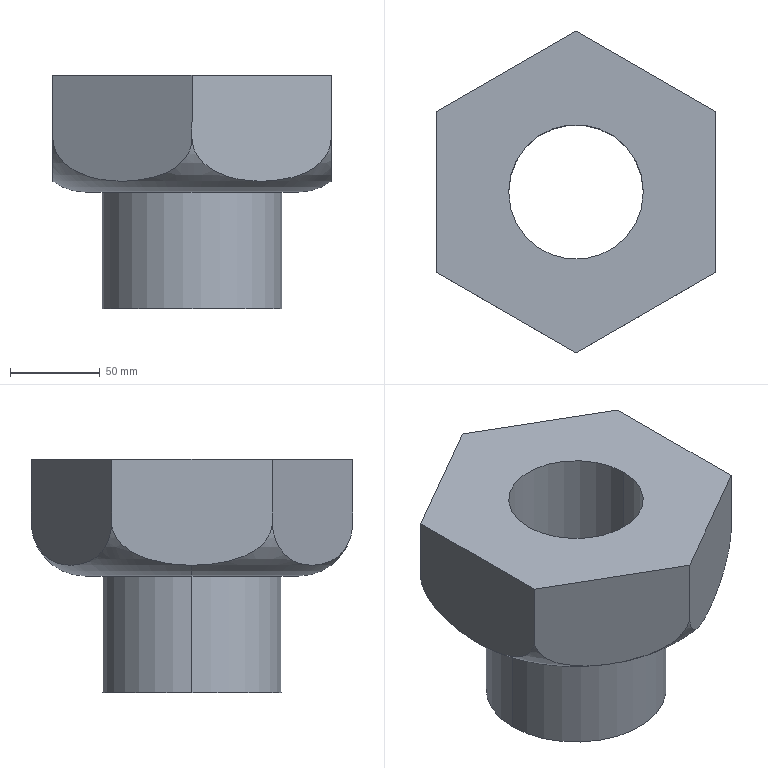Part | SolidWorks | features ICE 2, Extrusion 1, RevCut 1 | 1 solid | 15 faces | box 155 x 178.979 x 130 mm | volume 1254035 mm3 | plane 9 | cylinder 4 | torus 2 | commonest cylinder face diameters 75 x2 100 x2
STEP:
#1=CARTESIAN_POINT('',(37.5,0.,-65.));
#2=VERTEX_POINT('',#1);
#3=CARTESIAN_POINT('',(-37.5,0.,-65.));
#4=VERTEX_POINT('',#3);
#5=CARTESIAN_POINT('',(0.,0.,-65.));
#6=DIRECTION('',(0.,0.,-1.));
#7=DIRECTION('',(-1.,0.,0.));
#8=AXIS2_PLACEMENT_3D('',#5,#6,#7);
#9=CIRCLE('',#8,37.5);
#10=EDGE_CURVE('',#2,#4,#9,.T.);
#11=ORIENTED_EDGE('',*,*,#10,.T.);
#12=CARTESIAN_POINT('',(-37.5,0.,65.));
#13=VERTEX_POINT('',#12);
#14=CARTESIAN_POINT('',(-37.5,0.,-65.));
#15=DIRECTION('',(0.,0.,1.));
#16=VECTOR('',#15,1000.);
#17=LINE('',#14,#16);
#18=EDGE_CURVE('',#4,#13,#17,.T.);
#19=ORIENTED_EDGE('',*,*,#18,.T.);
#20=CARTESIAN_POINT('',(37.5,0.,65.));
#21=VERTEX_POINT('',#20);
#22=CARTESIAN_POINT('',(0.,0.,65.));
#23=DIRECTION('',(0.,0.,1.));
#24=DIRECTION('',(1.,0.,0.));
#25=AXIS2_PLACEMENT_3D('',#22,#23,#24);
#26=CIRCLE('',#25,37.5);
#27=EDGE_CURVE('',#13,#21,#26,.T.);
#28=ORIENTED_EDGE('',*,*,#27,.T.);
#29=CARTESIAN_POINT('',(37.5,0.,-65.));
#30=DIRECTION('',(0.,0.,1.));
#31=VECTOR('',#30,1000.);
#32=LINE('',#29,#31);
#33=EDGE_CURVE('',#2,#21,#32,.T.);
#34=ORIENTED_EDGE('',*,*,#33,.F.);
#35=EDGE_LOOP('',(#11,#19,#28,#34));
#36=FACE_OUTER_BOUND('',#35,.T.);
#37=CARTESIAN_POINT('',(0.,0.,-65.));
#38=DIRECTION('',(0.,0.,1.));
#39=DIRECTION('',(1.,0.,0.));
#40=AXIS2_PLACEMENT_3D('',#37,#38,#39);
#41=CYLINDRICAL_SURFACE('',#40,37.5);
#42=ADVANCED_FACE('',(#36),#41,.F.);
#43=CARTESIAN_POINT('',(-50.,0.,-65.));
#44=VERTEX_POINT('',#43);
#45=CARTESIAN_POINT('',(50.,0.,-65.));
#46=VERTEX_POINT('',#45);
#47=CARTESIAN_POINT('',(0.,0.,-65.));
#48=DIRECTION('',(0.,0.,-1.));
#49=DIRECTION('',(-1.,0.,0.));
#50=AXIS2_PLACEMENT_3D('',#47,#48,#49);
#51=CIRCLE('',#50,50.);
#52=EDGE_CURVE('',#44,#46,#51,.T.);
#53=ORIENTED_EDGE('',*,*,#52,.F.);
#54=CARTESIAN_POINT('',(-50.,0.,0.));
#55=VERTEX_POINT('',#54);
#56=CARTESIAN_POINT('',(-50.,0.,-65.));
#57=DIRECTION('',(0.,0.,1.));
#58=VECTOR('',#57,1000.);
#59=LINE('',#56,#58);
#60=EDGE_CURVE('',#44,#55,#59,.T.);
#61=ORIENTED_EDGE('',*,*,#60,.T.);
#62=CARTESIAN_POINT('',(50.,0.,0.));
#63=VERTEX_POINT('',#62);
#64=CARTESIAN_POINT('',(0.,0.,0.));
#65=DIRECTION('',(0.,0.,-1.));
#66=DIRECTION('',(1.,0.,0.));
#67=AXIS2_PLACEMENT_3D('',#64,#65,#66);
#68=CIRCLE('',#67,50.);
#69=EDGE_CURVE('',#55,#63,#68,.T.);
#70=ORIENTED_EDGE('',*,*,#69,.T.);
#71=CARTESIAN_POINT('',(50.,0.,-65.));
#72=DIRECTION('',(0.,0.,1.));
#73=VECTOR('',#72,1000.);
#74=LINE('',#71,#73);
#75=EDGE_CURVE('',#46,#63,#74,.T.);
#76=ORIENTED_EDGE('',*,*,#75,.F.);
#77=EDGE_LOOP('',(#53,#61,#70,#76));
#78=FACE_OUTER_BOUND('',#77,.T.);
#79=CARTESIAN_POINT('',(0.,0.,-65.));
#80=DIRECTION('',(0.,0.,1.));
#81=DIRECTION('',(1.,0.,0.));
#82=AXIS2_PLACEMENT_3D('',#79,#80,#81);
#83=CYLINDRICAL_SURFACE('',#82,50.);
#84=ADVANCED_FACE('',(#78),#83,.T.);
#85=CARTESIAN_POINT('',(59.489,0.,0.));
#86=VERTEX_POINT('',#85);
#87=CARTESIAN_POINT('',(-59.489,0.,0.));
#88=VERTEX_POINT('',#87);
#89=CARTESIAN_POINT('',(0.,0.,0.));
#90=DIRECTION('',(0.,0.,1.));
#91=DIRECTION('',(1.,0.,0.));
#92=AXIS2_PLACEMENT_3D('',#89,#90,#91);
#93=CIRCLE('',#92,59.489);
#94=EDGE_CURVE('',#86,#88,#93,.T.);
#95=ORIENTED_EDGE('',*,*,#94,.T.);
#96=CARTESIAN_POINT('',(-77.5,0.,6.008));
#97=VERTEX_POINT('',#96);
#98=CARTESIAN_POINT('',(-59.489,0.,30.));
#99=DIRECTION('',(0.,1.,0.));
#100=DIRECTION('',(-1.,0.,0.));
#101=AXIS2_PLACEMENT_3D('',#98,#99,#100);
#102=CIRCLE('',#101,30.);
#103=EDGE_CURVE('',#88,#97,#102,.T.);
#104=ORIENTED_EDGE('',*,*,#103,.T.);
#105=CARTESIAN_POINT('',(-77.5,44.745,30.));
#106=VERTEX_POINT('',#105);
#107=CARTESIAN_POINT('',(-77.5,0.,6.008));
#108=CARTESIAN_POINT('',(-77.5,2.326,6.008));
#109=CARTESIAN_POINT('',(-77.5,4.641,6.086));
#110=CARTESIAN_POINT('',(-77.5,9.25,6.403));
#111=CARTESIAN_POINT('',(-77.5,11.544,6.643));
#112=CARTESIAN_POINT('',(-77.5,16.107,7.312));
#113=CARTESIAN_POINT('',(-77.5,18.376,7.742));
#114=CARTESIAN_POINT('',(-77.5,21.755,8.571));
#115=CARTESIAN_POINT('',(-77.5,22.878,8.879));
#116=CARTESIAN_POINT('',(-77.5,25.11,9.566));
#117=CARTESIAN_POINT('',(-77.5,26.212,9.944));
#118=CARTESIAN_POINT('',(-77.5,28.383,10.777));
#119=CARTESIAN_POINT('',(-77.5,29.453,11.232));
#120=CARTESIAN_POINT('',(-77.5,31.028,11.984));
#121=CARTESIAN_POINT('',(-77.5,31.548,12.246));
#122=CARTESIAN_POINT('',(-77.5,32.578,12.795));
#123=CARTESIAN_POINT('',(-77.5,33.089,13.083));
#124=CARTESIAN_POINT('',(-77.5,34.59,13.98));
#125=CARTESIAN_POINT('',(-77.5,35.553,14.624));
#126=CARTESIAN_POINT('',(-77.5,37.393,16.021));
#127=CARTESIAN_POINT('',(-77.5,38.27,16.773));
#128=CARTESIAN_POINT('',(-77.5,39.506,17.998));
#129=CARTESIAN_POINT('',(-77.5,39.905,18.422));
#130=CARTESIAN_POINT('',(-77.5,40.673,19.309));
#131=CARTESIAN_POINT('',(-77.5,41.04,19.769));
#132=CARTESIAN_POINT('',(-77.5,42.074,21.184));
#133=CARTESIAN_POINT('',(-77.5,42.676,22.179));
#134=CARTESIAN_POINT('',(-77.5,43.43,23.763));
#135=CARTESIAN_POINT('',(-77.5,43.657,24.31));
#136=CARTESIAN_POINT('',(-77.5,44.047,25.415));
#137=CARTESIAN_POINT('',(-77.5,44.21,25.973));
#138=CARTESIAN_POINT('',(-77.5,44.607,27.667));
#139=CARTESIAN_POINT('',(-77.5,44.745,28.82));
#140=CARTESIAN_POINT('',(-77.5,44.745,30.));
#141=B_SPLINE_CURVE_WITH_KNOTS('',3,(#107,#108,#109,#110,#111,#112,#113,#114,#115,#116,#117,#118,#119,#120,#121,#122,#123,#124,#125,#126,#127,#128,#129,#130,#131,#132,#133,#134,#135,#136,#137,#138,#139,#140),.UNSPECIFIED.,.F.,.F.,(4,2,2,2,2,2,2,2,2,2,2,2,2,2,2,2,4),(0.,0.006917,0.01383,0.02075,0.02421,0.02767,0.03113,0.03285,0.03458,0.03804,0.0415,0.04323,0.04496,0.04842,0.05015,0.05188,0.05533),.UNSPECIFIED.);
#142=EDGE_CURVE('',#97,#106,#141,.T.);
#143=ORIENTED_EDGE('',*,*,#142,.T.);
#144=CARTESIAN_POINT('',(0.,89.489,30.));
#145=VERTEX_POINT('',#144);
#146=CARTESIAN_POINT('',(-77.5,44.745,30.));
#147=CARTESIAN_POINT('',(-77.5,44.745,28.82));
#148=CARTESIAN_POINT('',(-77.38,44.814,27.664));
#149=CARTESIAN_POINT('',(-77.035,45.013,25.963));
#150=CARTESIAN_POINT('',(-76.892,45.096,25.402));
#151=CARTESIAN_POINT('',(-76.551,45.292,24.291));
#152=CARTESIAN_POINT('',(-76.356,45.405,23.75));
#153=CARTESIAN_POINT('',(-75.704,45.782,22.169));
#154=CARTESIAN_POINT('',(-75.18,46.084,21.171));
#155=CARTESIAN_POINT('',(-73.975,46.78,19.271));
#156=CARTESIAN_POINT('',(-73.311,47.163,18.395));
#157=CARTESIAN_POINT('',(-71.883,47.988,16.763));
#158=CARTESIAN_POINT('',(-71.119,48.429,16.007));
#159=CARTESIAN_POINT('',(-69.909,49.127,14.949));
#160=CARTESIAN_POINT('',(-69.494,49.367,14.608));
#161=CARTESIAN_POINT('',(-68.653,49.852,13.958));
#162=CARTESIAN_POINT('',(-68.227,50.099,13.648));
#163=CARTESIAN_POINT('',(-66.066,51.346,12.163));
#164=CARTESIAN_POINT('',(-64.251,52.394,11.184));
#165=CARTESIAN_POINT('',(-61.436,54.019,9.938));
#166=CARTESIAN_POINT('',(-60.479,54.571,9.56));
#167=CARTESIAN_POINT('',(-58.55,55.686,8.874));
#168=CARTESIAN_POINT('',(-57.58,56.245,8.568));
#169=CARTESIAN_POINT('',(-54.66,57.931,7.741));
#170=CARTESIAN_POINT('',(-52.697,59.064,7.312));
#171=CARTESIAN_POINT('',(-48.749,61.344,6.643));
#172=CARTESIAN_POINT('',(-46.763,62.491,6.403));
#173=CARTESIAN_POINT('',(-43.769,64.22,6.165));
#174=CARTESIAN_POINT('',(-42.768,64.797,6.106));
#175=CARTESIAN_POINT('',(-40.761,65.956,6.028));
#176=CARTESIAN_POINT('',(-39.754,66.537,6.008));
#177=CARTESIAN_POINT('',(-36.741,68.277,6.008));
#178=CARTESIAN_POINT('',(-34.74,69.432,6.085));
#179=CARTESIAN_POINT('',(-30.759,71.731,6.401));
#180=CARTESIAN_POINT('',(-28.777,72.875,6.639));
#181=CARTESIAN_POINT('',(-24.836,75.15,7.305));
#182=CARTESIAN_POINT('',(-22.877,76.282,7.732));
#183=CARTESIAN_POINT('',(-19.958,77.966,8.556));
#184=CARTESIAN_POINT('',(-18.989,78.526,8.862));
#185=CARTESIAN_POINT('',(-17.059,79.64,9.545));
#186=CARTESIAN_POINT('',(-16.099,80.195,9.924));
#187=CARTESIAN_POINT('',(-14.213,81.284,10.756));
#188=CARTESIAN_POINT('',(-13.285,81.819,11.211));
#189=CARTESIAN_POINT('',(-11.918,82.608,11.961));
#190=CARTESIAN_POINT('',(-11.467,82.869,12.223));
#191=CARTESIAN_POINT('',(-10.574,83.385,12.771));
#192=CARTESIAN_POINT('',(-10.131,83.64,13.058));
#193=CARTESIAN_POINT('',(-8.827,84.393,13.955));
#194=CARTESIAN_POINT('',(-7.99,84.876,14.6));
#195=CARTESIAN_POINT('',(-6.389,85.8,15.999));
#196=CARTESIAN_POINT('',(-5.626,86.241,16.753));
#197=CARTESIAN_POINT('',(-4.549,86.863,17.983));
#198=CARTESIAN_POINT('',(-4.2,87.064,18.411));
#199=CARTESIAN_POINT('',(-3.535,87.448,19.297));
#200=CARTESIAN_POINT('',(-3.219,87.631,19.753));
#201=CARTESIAN_POINT('',(-2.326,88.146,21.162));
#202=CARTESIAN_POINT('',(-1.802,88.449,22.156));
#203=CARTESIAN_POINT('',(-1.146,88.828,23.745));
#204=CARTESIAN_POINT('',(-0.9494,88.941,24.289));
#205=CARTESIAN_POINT('',(-0.6116,89.136,25.389));
#206=CARTESIAN_POINT('',(-0.4689,89.219,25.947));
#207=CARTESIAN_POINT('',(-0.2379,89.352,27.079));
#208=CARTESIAN_POINT('',(-0.1495,89.403,27.653));
#209=CARTESIAN_POINT('',(-0.03038,89.472,28.819));
#210=CARTESIAN_POINT('',(0.,89.489,29.41));
#211=CARTESIAN_POINT('',(0.,89.489,30.));
#212=B_SPLINE_CURVE_WITH_KNOTS('',3,(#146,#147,#148,#149,#150,#151,#152,#153,#154,#155,#156,#157,#158,#159,#160,#161,#162,#163,#164,#165,#166,#167,#168,#169,#170,#171,#172,#173,#174,#175,#176,#177,#178,#179,#180,#181,#182,#183,#184,#185,#186,#187,#188,#189,#190,#191,#192,#193,#194,#195,#196,#197,#198,#199,#200,#201,#202,#203,#204,#205,#206,#207,#208,#209,#210,#211),.UNSPECIFIED.,.F.,.F.,(4,2,2,2,2,2,2,2,2,2,2,2,2,2,2,2,2,2,2,2,2,2,2,2,2,2,2,2,2,2,2,2,4),(0.000000197,0.003488,0.005232,0.006975,0.01046,0.01395,0.01744,0.01918,0.02093,0.0279,0.03139,0.03488,0.04185,0.04883,0.05231,0.0558,0.06278,0.06975,0.07673,0.08021,0.0837,0.08719,0.08893,0.09068,0.09417,0.09765,0.0994,0.1011,0.1046,0.1064,0.1081,0.1099,0.1116),.UNSPECIFIED.);
#213=EDGE_CURVE('',#106,#145,#212,.T.);
#214=ORIENTED_EDGE('',*,*,#213,.T.);
#215=CARTESIAN_POINT('',(77.5,44.745,30.));
#216=VERTEX_POINT('',#215);
#217=CARTESIAN_POINT('',(0.,89.489,30.));
#218=CARTESIAN_POINT('',(0.,89.489,28.82));
#219=CARTESIAN_POINT('',(0.1197,89.42,27.664));
#220=CARTESIAN_POINT('',(0.465,89.221,25.963));
#221=CARTESIAN_POINT('',(0.6079,89.138,25.402));
#222=CARTESIAN_POINT('',(0.9488,88.942,24.291));
#223=CARTESIAN_POINT('',(1.144,88.829,23.75));
#224=CARTESIAN_POINT('',(1.796,88.452,22.169));
#225=CARTESIAN_POINT('',(2.32,88.15,21.171));
#226=CARTESIAN_POINT('',(3.525,87.454,19.271));
#227=CARTESIAN_POINT('',(4.189,87.071,18.395));
#228=CARTESIAN_POINT('',(5.617,86.246,16.763));
#229=CARTESIAN_POINT('',(6.381,85.805,16.007));
#230=CARTESIAN_POINT('',(7.591,85.107,14.949));
#231=CARTESIAN_POINT('',(8.006,84.867,14.608));
#232=CARTESIAN_POINT('',(8.847,84.382,13.958));
#233=CARTESIAN_POINT('',(9.273,84.135,13.648));
#234=CARTESIAN_POINT('',(11.434,82.888,12.163));
#235=CARTESIAN_POINT('',(13.249,81.84,11.184));
#236=CARTESIAN_POINT('',(16.064,80.215,9.938));
#237=CARTESIAN_POINT('',(17.021,79.662,9.56));
#238=CARTESIAN_POINT('',(18.95,78.548,8.874));
#239=CARTESIAN_POINT('',(19.92,77.988,8.568));
#240=CARTESIAN_POINT('',(22.84,76.302,7.741));
#241=CARTESIAN_POINT('',(24.803,75.17,7.312));
#242=CARTESIAN_POINT('',(28.751,72.89,6.643));
#243=CARTESIAN_POINT('',(30.737,71.743,6.403));
#244=CARTESIAN_POINT('',(33.731,70.014,6.165));
#245=CARTESIAN_POINT('',(34.732,69.437,6.106));
#246=CARTESIAN_POINT('',(36.739,68.278,6.028));
#247=CARTESIAN_POINT('',(37.746,67.697,6.008));
#248=CARTESIAN_POINT('',(40.759,65.957,6.008));
#249=CARTESIAN_POINT('',(42.76,64.802,6.085));
#250=CARTESIAN_POINT('',(46.741,62.503,6.401));
#251=CARTESIAN_POINT('',(48.723,61.359,6.639));
#252=CARTESIAN_POINT('',(52.664,59.084,7.305));
#253=CARTESIAN_POINT('',(54.623,57.952,7.732));
#254=CARTESIAN_POINT('',(57.542,56.268,8.556));
#255=CARTESIAN_POINT('',(58.511,55.708,8.862));
#256=CARTESIAN_POINT('',(60.441,54.594,9.545));
#257=CARTESIAN_POINT('',(61.401,54.039,9.924));
#258=CARTESIAN_POINT('',(63.287,52.95,10.756));
#259=CARTESIAN_POINT('',(64.215,52.415,11.211));
#260=CARTESIAN_POINT('',(65.582,51.625,11.961));
#261=CARTESIAN_POINT('',(66.033,51.365,12.223));
#262=CARTESIAN_POINT('',(66.926,50.849,12.771));
#263=CARTESIAN_POINT('',(67.369,50.594,13.058));
#264=CARTESIAN_POINT('',(68.673,49.841,13.955));
#265=CARTESIAN_POINT('',(69.51,49.358,14.6));
#266=CARTESIAN_POINT('',(71.111,48.434,15.999));
#267=CARTESIAN_POINT('',(71.874,47.993,16.753));
#268=CARTESIAN_POINT('',(72.951,47.371,17.983));
#269=CARTESIAN_POINT('',(73.3,47.17,18.411));
#270=CARTESIAN_POINT('',(73.965,46.786,19.297));
#271=CARTESIAN_POINT('',(74.281,46.603,19.753));
#272=CARTESIAN_POINT('',(75.174,46.088,21.162));
#273=CARTESIAN_POINT('',(75.698,45.785,22.156));
#274=CARTESIAN_POINT('',(76.354,45.406,23.745));
#275=CARTESIAN_POINT('',(76.551,45.293,24.289));
#276=CARTESIAN_POINT('',(76.888,45.098,25.389));
#277=CARTESIAN_POINT('',(77.031,45.015,25.947));
#278=CARTESIAN_POINT('',(77.262,44.882,27.079));
#279=CARTESIAN_POINT('',(77.35,44.831,27.653));
#280=CARTESIAN_POINT('',(77.47,44.762,28.819));
#281=CARTESIAN_POINT('',(77.5,44.745,29.41));
#282=CARTESIAN_POINT('',(77.5,44.745,30.));
#283=B_SPLINE_CURVE_WITH_KNOTS('',3,(#217,#218,#219,#220,#221,#222,#223,#224,#225,#226,#227,#228,#229,#230,#231,#232,#233,#234,#235,#236,#237,#238,#239,#240,#241,#242,#243,#244,#245,#246,#247,#248,#249,#250,#251,#252,#253,#254,#255,#256,#257,#258,#259,#260,#261,#262,#263,#264,#265,#266,#267,#268,#269,#270,#271,#272,#273,#274,#275,#276,#277,#278,#279,#280,#281,#282),.UNSPECIFIED.,.F.,.F.,(4,2,2,2,2,2,2,2,2,2,2,2,2,2,2,2,2,2,2,2,2,2,2,2,2,2,2,2,2,2,2,2,4),(0.000000197,0.003488,0.005232,0.006975,0.01046,0.01395,0.01744,0.01918,0.02093,0.0279,0.03139,0.03488,0.04185,0.04883,0.05231,0.0558,0.06278,0.06975,0.07673,0.08021,0.0837,0.08719,0.08893,0.09068,0.09417,0.09765,0.0994,0.1011,0.1046,0.1064,0.1081,0.1099,0.1116),.UNSPECIFIED.);
#284=EDGE_CURVE('',#145,#216,#283,.T.);
#285=ORIENTED_EDGE('',*,*,#284,.T.);
#286=CARTESIAN_POINT('',(77.5,0.,6.008));
#287=VERTEX_POINT('',#286);
#288=CARTESIAN_POINT('',(77.5,44.745,30.));
#289=CARTESIAN_POINT('',(77.5,44.745,29.421));
#290=CARTESIAN_POINT('',(77.5,44.711,28.842));
#291=CARTESIAN_POINT('',(77.5,44.576,27.68));
#292=CARTESIAN_POINT('',(77.5,44.474,27.097));
#293=CARTESIAN_POINT('',(77.5,44.073,25.391));
#294=CARTESIAN_POINT('',(77.5,43.682,24.295));
#295=CARTESIAN_POINT('',(77.5,42.927,22.706));
#296=CARTESIAN_POINT('',(77.5,42.647,22.187));
#297=CARTESIAN_POINT('',(77.5,42.046,21.188));
#298=CARTESIAN_POINT('',(77.5,41.724,20.705));
#299=CARTESIAN_POINT('',(77.5,40.698,19.3));
#300=CARTESIAN_POINT('',(77.5,39.934,18.423));
#301=CARTESIAN_POINT('',(77.5,38.686,17.185));
#302=CARTESIAN_POINT('',(77.5,38.255,16.788));
#303=CARTESIAN_POINT('',(77.5,37.374,16.028));
#304=CARTESIAN_POINT('',(77.5,36.923,15.663));
#305=CARTESIAN_POINT('',(77.5,35.538,14.614));
#306=CARTESIAN_POINT('',(77.5,34.576,13.971));
#307=CARTESIAN_POINT('',(77.5,33.084,13.08));
#308=CARTESIAN_POINT('',(77.5,32.578,12.795));
#309=CARTESIAN_POINT('',(77.5,31.551,12.247));
#310=CARTESIAN_POINT('',(77.5,31.028,11.984));
#311=CARTESIAN_POINT('',(77.5,29.449,11.23));
#312=CARTESIAN_POINT('',(77.5,28.381,10.776));
#313=CARTESIAN_POINT('',(77.5,25.143,9.533));
#314=CARTESIAN_POINT('',(77.5,22.936,8.863));
#315=CARTESIAN_POINT('',(77.5,19.574,8.034));
#316=CARTESIAN_POINT('',(77.5,18.445,7.788));
#317=CARTESIAN_POINT('',(77.5,16.17,7.348));
#318=CARTESIAN_POINT('',(77.5,15.023,7.154));
#319=CARTESIAN_POINT('',(77.5,11.575,6.646));
#320=CARTESIAN_POINT('',(77.5,9.268,6.405));
#321=CARTESIAN_POINT('',(77.5,5.8,6.165));
#322=CARTESIAN_POINT('',(77.5,4.642,6.106));
#323=CARTESIAN_POINT('',(77.5,2.903,6.047));
#324=CARTESIAN_POINT('',(77.5,2.323,6.033));
#325=CARTESIAN_POINT('',(77.5,1.452,6.018));
#326=CARTESIAN_POINT('',(77.5,1.162,6.014));
#327=CARTESIAN_POINT('',(77.5,0.5811,6.009));
#328=CARTESIAN_POINT('',(77.5,0.2891,6.008));
#329=CARTESIAN_POINT('',(77.5,0.,6.008));
#330=B_SPLINE_CURVE_WITH_KNOTS('',3,(#288,#289,#290,#291,#292,#293,#294,#295,#296,#297,#298,#299,#300,#301,#302,#303,#304,#305,#306,#307,#308,#309,#310,#311,#312,#313,#314,#315,#316,#317,#318,#319,#320,#321,#322,#323,#324,#325,#326,#327,#328,#329),.UNSPECIFIED.,.F.,.F.,(4,2,2,2,2,2,2,2,2,2,2,2,2,2,2,2,2,2,2,2,4),(0.1659,0.1677,0.1694,0.1728,0.1745,0.1763,0.1797,0.1814,0.1831,0.1866,0.1883,0.19,0.1935,0.2003,0.2038,0.2072,0.2141,0.2175,0.2192,0.2201,0.221),.UNSPECIFIED.);
#331=EDGE_CURVE('',#216,#287,#330,.T.);
#332=ORIENTED_EDGE('',*,*,#331,.T.);
#333=CARTESIAN_POINT('',(59.489,0.,30.));
#334=DIRECTION('',(0.,-1.,0.));
#335=DIRECTION('',(0.,0.,-1.));
#336=AXIS2_PLACEMENT_3D('',#333,#334,#335);
#337=CIRCLE('',#336,30.);
#338=EDGE_CURVE('',#86,#287,#337,.T.);
#339=ORIENTED_EDGE('',*,*,#338,.F.);
#340=EDGE_LOOP('',(#95,#104,#143,#214,#285,#332,#339));
#341=FACE_OUTER_BOUND('',#340,.T.);
#342=CARTESIAN_POINT('',(0.,0.,30.));
#343=DIRECTION('',(0.,0.,1.));
#344=DIRECTION('',(1.,0.,0.));
#345=AXIS2_PLACEMENT_3D('',#342,#343,#344);
#346=TOROIDAL_SURFACE('',#345,59.489,30.);
#347=ADVANCED_FACE('',(#341),#346,.T.);
#348=ORIENTED_EDGE('',*,*,#94,.F.);
#349=CARTESIAN_POINT('',(0.,0.,0.));
#350=DIRECTION('',(0.,0.,1.));
#351=DIRECTION('',(1.,0.,0.));
#352=AXIS2_PLACEMENT_3D('',#349,#350,#351);
#353=CIRCLE('',#352,59.489);
#354=EDGE_CURVE('',#88,#86,#353,.T.);
#355=ORIENTED_EDGE('',*,*,#354,.F.);
#356=EDGE_LOOP('',(#348,#355));
#357=FACE_OUTER_BOUND('',#356,.T.);
#358=CARTESIAN_POINT('',(0.,0.,0.));
#359=DIRECTION('',(0.,0.,-1.));
#360=DIRECTION('',(1.,0.,0.));
#361=AXIS2_PLACEMENT_3D('',#358,#359,#360);
#362=CIRCLE('',#361,50.);
#363=EDGE_CURVE('',#63,#55,#362,.T.);
#364=ORIENTED_EDGE('',*,*,#363,.F.);
#365=ORIENTED_EDGE('',*,*,#69,.F.);
#366=EDGE_LOOP('',(#364,#365));
#367=FACE_BOUND('',#366,.T.);
#368=CARTESIAN_POINT('',(0.,0.,0.));
#369=DIRECTION('',(0.,0.,1.));
#370=DIRECTION('',(1.,0.,0.));
#371=AXIS2_PLACEMENT_3D('',#368,#369,#370);
#372=PLANE('',#371);
#373=ADVANCED_FACE('',(#357,#367),#372,.F.);
#374=ORIENTED_EDGE('',*,*,#331,.F.);
#375=CARTESIAN_POINT('',(77.5,44.745,65.));
#376=VERTEX_POINT('',#375);
#377=CARTESIAN_POINT('',(77.5,44.745,65.));
#378=DIRECTION('',(0.,0.,-1.));
#379=VECTOR('',#378,1000.);
#380=LINE('',#377,#379);
#381=EDGE_CURVE('',#376,#216,#380,.T.);
#382=ORIENTED_EDGE('',*,*,#381,.F.);
#383=CARTESIAN_POINT('',(77.5,-44.745,65.));
#384=VERTEX_POINT('',#383);
#385=CARTESIAN_POINT('',(77.5,-44.745,65.));
#386=DIRECTION('',(0.,1.,0.));
#387=VECTOR('',#386,1000.);
#388=LINE('',#385,#387);
#389=EDGE_CURVE('',#384,#376,#388,.T.);
#390=ORIENTED_EDGE('',*,*,#389,.F.);
#391=CARTESIAN_POINT('',(77.5,-44.745,30.));
#392=VERTEX_POINT('',#391);
#393=CARTESIAN_POINT('',(77.5,-44.745,65.));
#394=DIRECTION('',(0.,0.,-1.));
#395=VECTOR('',#394,1000.);
#396=LINE('',#393,#395);
#397=EDGE_CURVE('',#384,#392,#396,.T.);
#398=ORIENTED_EDGE('',*,*,#397,.T.);
#399=CARTESIAN_POINT('',(77.5,0.,6.008));
#400=CARTESIAN_POINT('',(77.5,-2.326,6.008));
#401=CARTESIAN_POINT('',(77.5,-4.641,6.086));
#402=CARTESIAN_POINT('',(77.5,-9.25,6.403));
#403=CARTESIAN_POINT('',(77.5,-11.544,6.643));
#404=CARTESIAN_POINT('',(77.5,-16.107,7.312));
#405=CARTESIAN_POINT('',(77.5,-18.376,7.742));
#406=CARTESIAN_POINT('',(77.5,-21.755,8.571));
#407=CARTESIAN_POINT('',(77.5,-22.878,8.879));
#408=CARTESIAN_POINT('',(77.5,-25.11,9.566));
#409=CARTESIAN_POINT('',(77.5,-26.212,9.944));
#410=CARTESIAN_POINT('',(77.5,-28.383,10.777));
#411=CARTESIAN_POINT('',(77.5,-29.453,11.232));
#412=CARTESIAN_POINT('',(77.5,-31.028,11.984));
#413=CARTESIAN_POINT('',(77.5,-31.548,12.246));
#414=CARTESIAN_POINT('',(77.5,-32.578,12.795));
#415=CARTESIAN_POINT('',(77.5,-33.089,13.083));
#416=CARTESIAN_POINT('',(77.5,-34.59,13.98));
#417=CARTESIAN_POINT('',(77.5,-35.553,14.624));
#418=CARTESIAN_POINT('',(77.5,-37.393,16.021));
#419=CARTESIAN_POINT('',(77.5,-38.27,16.773));
#420=CARTESIAN_POINT('',(77.5,-39.506,17.998));
#421=CARTESIAN_POINT('',(77.5,-39.905,18.422));
#422=CARTESIAN_POINT('',(77.5,-40.673,19.309));
#423=CARTESIAN_POINT('',(77.5,-41.04,19.769));
#424=CARTESIAN_POINT('',(77.5,-42.074,21.184));
#425=CARTESIAN_POINT('',(77.5,-42.676,22.179));
#426=CARTESIAN_POINT('',(77.5,-43.43,23.763));
#427=CARTESIAN_POINT('',(77.5,-43.657,24.31));
#428=CARTESIAN_POINT('',(77.5,-44.047,25.415));
#429=CARTESIAN_POINT('',(77.5,-44.21,25.973));
#430=CARTESIAN_POINT('',(77.5,-44.607,27.667));
#431=CARTESIAN_POINT('',(77.5,-44.745,28.82));
#432=CARTESIAN_POINT('',(77.5,-44.745,30.));
#433=B_SPLINE_CURVE_WITH_KNOTS('',3,(#399,#400,#401,#402,#403,#404,#405,#406,#407,#408,#409,#410,#411,#412,#413,#414,#415,#416,#417,#418,#419,#420,#421,#422,#423,#424,#425,#426,#427,#428,#429,#430,#431,#432),.UNSPECIFIED.,.F.,.F.,(4,2,2,2,2,2,2,2,2,2,2,2,2,2,2,2,4),(0.,0.006917,0.01383,0.02075,0.02421,0.02767,0.03113,0.03285,0.03458,0.03804,0.0415,0.04323,0.04496,0.04842,0.05015,0.05188,0.05533),.UNSPECIFIED.);
#434=EDGE_CURVE('',#287,#392,#433,.T.);
#435=ORIENTED_EDGE('',*,*,#434,.F.);
#436=EDGE_LOOP('',(#374,#382,#390,#398,#435));
#437=FACE_OUTER_BOUND('',#436,.T.);
#438=CARTESIAN_POINT('',(77.5,-44.745,65.));
#439=DIRECTION('',(-1.,0.,0.));
#440=DIRECTION('',(0.,-1.,0.));
#441=AXIS2_PLACEMENT_3D('',#438,#439,#440);
#442=PLANE('',#441);
#443=ADVANCED_FACE('',(#437),#442,.F.);
#444=ORIENTED_EDGE('',*,*,#284,.F.);
#445=CARTESIAN_POINT('',(0.,89.489,65.));
#446=VERTEX_POINT('',#445);
#447=CARTESIAN_POINT('',(0.,89.489,65.));
#448=DIRECTION('',(0.,0.,-1.));
#449=VECTOR('',#448,1000.);
#450=LINE('',#447,#449);
#451=EDGE_CURVE('',#446,#145,#450,.T.);
#452=ORIENTED_EDGE('',*,*,#451,.F.);
#453=CARTESIAN_POINT('',(77.5,44.745,65.));
#454=DIRECTION('',(-0.866,0.5,0.));
#455=VECTOR('',#454,1000.);
#456=LINE('',#453,#455);
#457=EDGE_CURVE('',#376,#446,#456,.T.);
#458=ORIENTED_EDGE('',*,*,#457,.F.);
#459=ORIENTED_EDGE('',*,*,#381,.T.);
#460=EDGE_LOOP('',(#444,#452,#458,#459));
#461=FACE_OUTER_BOUND('',#460,.T.);
#462=CARTESIAN_POINT('',(77.5,44.745,65.));
#463=DIRECTION('',(-0.5,-0.866,0.));
#464=DIRECTION('',(0.866,-0.5,0.));
#465=AXIS2_PLACEMENT_3D('',#462,#463,#464);
#466=PLANE('',#465);
#467=ADVANCED_FACE('',(#461),#466,.F.);
#468=ORIENTED_EDGE('',*,*,#213,.F.);
#469=CARTESIAN_POINT('',(-77.5,44.745,65.));
#470=VERTEX_POINT('',#469);
#471=CARTESIAN_POINT('',(-77.5,44.745,65.));
#472=DIRECTION('',(0.,0.,-1.));
#473=VECTOR('',#472,1000.);
#474=LINE('',#471,#473);
#475=EDGE_CURVE('',#470,#106,#474,.T.);
#476=ORIENTED_EDGE('',*,*,#475,.F.);
#477=CARTESIAN_POINT('',(0.,89.489,65.));
#478=DIRECTION('',(-0.866,-0.5,0.));
#479=VECTOR('',#478,1000.);
#480=LINE('',#477,#479);
#481=EDGE_CURVE('',#446,#470,#480,.T.);
#482=ORIENTED_EDGE('',*,*,#481,.F.);
#483=ORIENTED_EDGE('',*,*,#451,.T.);
#484=EDGE_LOOP('',(#468,#476,#482,#483));
#485=FACE_OUTER_BOUND('',#484,.T.);
#486=CARTESIAN_POINT('',(0.,89.489,65.));
#487=DIRECTION('',(0.5,-0.866,0.));
#488=DIRECTION('',(0.866,0.5,0.));
#489=AXIS2_PLACEMENT_3D('',#486,#487,#488);
#490=PLANE('',#489);
#491=ADVANCED_FACE('',(#485),#490,.F.);
#492=CARTESIAN_POINT('',(-77.5,-44.745,30.));
#493=VERTEX_POINT('',#492);
#494=CARTESIAN_POINT('',(-77.5,-44.745,30.));
#495=CARTESIAN_POINT('',(-77.5,-44.745,29.421));
#496=CARTESIAN_POINT('',(-77.5,-44.711,28.842));
#497=CARTESIAN_POINT('',(-77.5,-44.576,27.68));
#498=CARTESIAN_POINT('',(-77.5,-44.474,27.097));
#499=CARTESIAN_POINT('',(-77.5,-44.073,25.391));
#500=CARTESIAN_POINT('',(-77.5,-43.682,24.295));
#501=CARTESIAN_POINT('',(-77.5,-42.927,22.706));
#502=CARTESIAN_POINT('',(-77.5,-42.647,22.187));
#503=CARTESIAN_POINT('',(-77.5,-42.046,21.188));
#504=CARTESIAN_POINT('',(-77.5,-41.724,20.705));
#505=CARTESIAN_POINT('',(-77.5,-40.698,19.3));
#506=CARTESIAN_POINT('',(-77.5,-39.934,18.423));
#507=CARTESIAN_POINT('',(-77.5,-38.686,17.185));
#508=CARTESIAN_POINT('',(-77.5,-38.255,16.788));
#509=CARTESIAN_POINT('',(-77.5,-37.374,16.028));
#510=CARTESIAN_POINT('',(-77.5,-36.923,15.663));
#511=CARTESIAN_POINT('',(-77.5,-35.538,14.614));
#512=CARTESIAN_POINT('',(-77.5,-34.576,13.971));
#513=CARTESIAN_POINT('',(-77.5,-33.084,13.08));
#514=CARTESIAN_POINT('',(-77.5,-32.578,12.795));
#515=CARTESIAN_POINT('',(-77.5,-31.551,12.247));
#516=CARTESIAN_POINT('',(-77.5,-31.028,11.984));
#517=CARTESIAN_POINT('',(-77.5,-29.449,11.23));
#518=CARTESIAN_POINT('',(-77.5,-28.381,10.776));
#519=CARTESIAN_POINT('',(-77.5,-25.143,9.533));
#520=CARTESIAN_POINT('',(-77.5,-22.936,8.863));
#521=CARTESIAN_POINT('',(-77.5,-19.574,8.034));
#522=CARTESIAN_POINT('',(-77.5,-18.445,7.788));
#523=CARTESIAN_POINT('',(-77.5,-16.17,7.348));
#524=CARTESIAN_POINT('',(-77.5,-15.023,7.154));
#525=CARTESIAN_POINT('',(-77.5,-11.575,6.646));
#526=CARTESIAN_POINT('',(-77.5,-9.268,6.405));
#527=CARTESIAN_POINT('',(-77.5,-5.8,6.165));
#528=CARTESIAN_POINT('',(-77.5,-4.642,6.106));
#529=CARTESIAN_POINT('',(-77.5,-2.903,6.047));
#530=CARTESIAN_POINT('',(-77.5,-2.323,6.033));
#531=CARTESIAN_POINT('',(-77.5,-1.452,6.018));
#532=CARTESIAN_POINT('',(-77.5,-1.162,6.014));
#533=CARTESIAN_POINT('',(-77.5,-0.5811,6.009));
#534=CARTESIAN_POINT('',(-77.5,-0.2891,6.008));
#535=CARTESIAN_POINT('',(-77.5,0.,6.008));
#536=B_SPLINE_CURVE_WITH_KNOTS('',3,(#494,#495,#496,#497,#498,#499,#500,#501,#502,#503,#504,#505,#506,#507,#508,#509,#510,#511,#512,#513,#514,#515,#516,#517,#518,#519,#520,#521,#522,#523,#524,#525,#526,#527,#528,#529,#530,#531,#532,#533,#534,#535),.UNSPECIFIED.,.F.,.F.,(4,2,2,2,2,2,2,2,2,2,2,2,2,2,2,2,2,2,2,2,4),(0.1659,0.1677,0.1694,0.1728,0.1745,0.1763,0.1797,0.1814,0.1831,0.1866,0.1883,0.19,0.1935,0.2003,0.2038,0.2072,0.2141,0.2175,0.2192,0.2201,0.221),.UNSPECIFIED.);
#537=EDGE_CURVE('',#493,#97,#536,.T.);
#538=ORIENTED_EDGE('',*,*,#537,.F.);
#539=CARTESIAN_POINT('',(-77.5,-44.745,65.));
#540=VERTEX_POINT('',#539);
#541=CARTESIAN_POINT('',(-77.5,-44.745,65.));
#542=DIRECTION('',(0.,0.,-1.));
#543=VECTOR('',#542,1000.);
#544=LINE('',#541,#543);
#545=EDGE_CURVE('',#540,#493,#544,.T.);
#546=ORIENTED_EDGE('',*,*,#545,.F.);
#547=CARTESIAN_POINT('',(-77.5,44.745,65.));
#548=DIRECTION('',(0.,-1.,0.));
#549=VECTOR('',#548,1000.);
#550=LINE('',#547,#549);
#551=EDGE_CURVE('',#470,#540,#550,.T.);
#552=ORIENTED_EDGE('',*,*,#551,.F.);
#553=ORIENTED_EDGE('',*,*,#475,.T.);
#554=ORIENTED_EDGE('',*,*,#142,.F.);
#555=EDGE_LOOP('',(#538,#546,#552,#553,#554));
#556=FACE_OUTER_BOUND('',#555,.T.);
#557=CARTESIAN_POINT('',(-77.5,44.745,65.));
#558=DIRECTION('',(1.,0.,0.));
#559=DIRECTION('',(0.,1.,0.));
#560=AXIS2_PLACEMENT_3D('',#557,#558,#559);
#561=PLANE('',#560);
#562=ADVANCED_FACE('',(#556),#561,.F.);
#563=CARTESIAN_POINT('',(0.,-89.489,30.));
#564=VERTEX_POINT('',#563);
#565=CARTESIAN_POINT('',(0.,-89.489,30.));
#566=CARTESIAN_POINT('',(0.,-89.489,28.82));
#567=CARTESIAN_POINT('',(-0.1197,-89.42,27.664));
#568=CARTESIAN_POINT('',(-0.465,-89.221,25.963));
#569=CARTESIAN_POINT('',(-0.6079,-89.138,25.402));
#570=CARTESIAN_POINT('',(-0.9488,-88.942,24.291));
#571=CARTESIAN_POINT('',(-1.144,-88.829,23.75));
#572=CARTESIAN_POINT('',(-1.796,-88.452,22.169));
#573=CARTESIAN_POINT('',(-2.32,-88.15,21.171));
#574=CARTESIAN_POINT('',(-3.525,-87.454,19.271));
#575=CARTESIAN_POINT('',(-4.189,-87.071,18.395));
#576=CARTESIAN_POINT('',(-5.617,-86.246,16.763));
#577=CARTESIAN_POINT('',(-6.381,-85.805,16.007));
#578=CARTESIAN_POINT('',(-7.591,-85.107,14.949));
#579=CARTESIAN_POINT('',(-8.006,-84.867,14.608));
#580=CARTESIAN_POINT('',(-8.847,-84.382,13.958));
#581=CARTESIAN_POINT('',(-9.273,-84.135,13.648));
#582=CARTESIAN_POINT('',(-11.434,-82.888,12.163));
#583=CARTESIAN_POINT('',(-13.249,-81.84,11.184));
#584=CARTESIAN_POINT('',(-16.064,-80.215,9.938));
#585=CARTESIAN_POINT('',(-17.021,-79.662,9.56));
#586=CARTESIAN_POINT('',(-18.95,-78.548,8.874));
#587=CARTESIAN_POINT('',(-19.92,-77.988,8.568));
#588=CARTESIAN_POINT('',(-22.84,-76.302,7.741));
#589=CARTESIAN_POINT('',(-24.803,-75.17,7.312));
#590=CARTESIAN_POINT('',(-28.751,-72.89,6.643));
#591=CARTESIAN_POINT('',(-30.737,-71.743,6.403));
#592=CARTESIAN_POINT('',(-33.731,-70.014,6.165));
#593=CARTESIAN_POINT('',(-34.732,-69.437,6.106));
#594=CARTESIAN_POINT('',(-36.739,-68.278,6.028));
#595=CARTESIAN_POINT('',(-37.746,-67.697,6.008));
#596=CARTESIAN_POINT('',(-40.759,-65.957,6.008));
#597=CARTESIAN_POINT('',(-42.76,-64.802,6.085));
#598=CARTESIAN_POINT('',(-46.741,-62.503,6.401));
#599=CARTESIAN_POINT('',(-48.723,-61.359,6.639));
#600=CARTESIAN_POINT('',(-52.664,-59.084,7.305));
#601=CARTESIAN_POINT('',(-54.623,-57.952,7.732));
#602=CARTESIAN_POINT('',(-57.542,-56.268,8.556));
#603=CARTESIAN_POINT('',(-58.511,-55.708,8.862));
#604=CARTESIAN_POINT('',(-60.441,-54.594,9.545));
#605=CARTESIAN_POINT('',(-61.401,-54.039,9.924));
#606=CARTESIAN_POINT('',(-63.287,-52.95,10.756));
#607=CARTESIAN_POINT('',(-64.215,-52.415,11.211));
#608=CARTESIAN_POINT('',(-65.582,-51.625,11.961));
#609=CARTESIAN_POINT('',(-66.033,-51.365,12.223));
#610=CARTESIAN_POINT('',(-66.926,-50.849,12.771));
#611=CARTESIAN_POINT('',(-67.369,-50.594,13.058));
#612=CARTESIAN_POINT('',(-68.673,-49.841,13.955));
#613=CARTESIAN_POINT('',(-69.51,-49.358,14.6));
#614=CARTESIAN_POINT('',(-71.111,-48.434,15.999));
#615=CARTESIAN_POINT('',(-71.874,-47.993,16.753));
#616=CARTESIAN_POINT('',(-72.951,-47.371,17.983));
#617=CARTESIAN_POINT('',(-73.3,-47.17,18.411));
#618=CARTESIAN_POINT('',(-73.965,-46.786,19.297));
#619=CARTESIAN_POINT('',(-74.281,-46.603,19.753));
#620=CARTESIAN_POINT('',(-75.174,-46.088,21.162));
#621=CARTESIAN_POINT('',(-75.698,-45.785,22.156));
#622=CARTESIAN_POINT('',(-76.354,-45.406,23.745));
#623=CARTESIAN_POINT('',(-76.551,-45.293,24.289));
#624=CARTESIAN_POINT('',(-76.888,-45.098,25.389));
#625=CARTESIAN_POINT('',(-77.031,-45.015,25.947));
#626=CARTESIAN_POINT('',(-77.262,-44.882,27.079));
#627=CARTESIAN_POINT('',(-77.35,-44.831,27.653));
#628=CARTESIAN_POINT('',(-77.47,-44.762,28.819));
#629=CARTESIAN_POINT('',(-77.5,-44.745,29.41));
#630=CARTESIAN_POINT('',(-77.5,-44.745,30.));
#631=B_SPLINE_CURVE_WITH_KNOTS('',3,(#565,#566,#567,#568,#569,#570,#571,#572,#573,#574,#575,#576,#577,#578,#579,#580,#581,#582,#583,#584,#585,#586,#587,#588,#589,#590,#591,#592,#593,#594,#595,#596,#597,#598,#599,#600,#601,#602,#603,#604,#605,#606,#607,#608,#609,#610,#611,#612,#613,#614,#615,#616,#617,#618,#619,#620,#621,#622,#623,#624,#625,#626,#627,#628,#629,#630),.UNSPECIFIED.,.F.,.F.,(4,2,2,2,2,2,2,2,2,2,2,2,2,2,2,2,2,2,2,2,2,2,2,2,2,2,2,2,2,2,2,2,4),(0.000000197,0.003488,0.005232,0.006975,0.01046,0.01395,0.01744,0.01918,0.02093,0.0279,0.03139,0.03488,0.04185,0.04883,0.05231,0.0558,0.06278,0.06975,0.07673,0.08021,0.0837,0.08719,0.08893,0.09068,0.09417,0.09765,0.0994,0.1011,0.1046,0.1064,0.1081,0.1099,0.1116),.UNSPECIFIED.);
#632=EDGE_CURVE('',#564,#493,#631,.T.);
#633=ORIENTED_EDGE('',*,*,#632,.F.);
#634=CARTESIAN_POINT('',(0.,-89.489,65.));
#635=VERTEX_POINT('',#634);
#636=CARTESIAN_POINT('',(0.,-89.489,65.));
#637=DIRECTION('',(0.,0.,-1.));
#638=VECTOR('',#637,1000.);
#639=LINE('',#636,#638);
#640=EDGE_CURVE('',#635,#564,#639,.T.);
#641=ORIENTED_EDGE('',*,*,#640,.F.);
#642=CARTESIAN_POINT('',(-77.5,-44.745,65.));
#643=DIRECTION('',(0.866,-0.5,0.));
#644=VECTOR('',#643,1000.);
#645=LINE('',#642,#644);
#646=EDGE_CURVE('',#540,#635,#645,.T.);
#647=ORIENTED_EDGE('',*,*,#646,.F.);
#648=ORIENTED_EDGE('',*,*,#545,.T.);
#649=EDGE_LOOP('',(#633,#641,#647,#648));
#650=FACE_OUTER_BOUND('',#649,.T.);
#651=CARTESIAN_POINT('',(-77.5,-44.745,65.));
#652=DIRECTION('',(0.5,0.866,0.));
#653=DIRECTION('',(-0.866,0.5,0.));
#654=AXIS2_PLACEMENT_3D('',#651,#652,#653);
#655=PLANE('',#654);
#656=ADVANCED_FACE('',(#650),#655,.F.);
#657=CARTESIAN_POINT('',(77.5,-44.745,30.));
#658=CARTESIAN_POINT('',(77.5,-44.745,28.82));
#659=CARTESIAN_POINT('',(77.38,-44.814,27.664));
#660=CARTESIAN_POINT('',(77.035,-45.013,25.963));
#661=CARTESIAN_POINT('',(76.892,-45.096,25.402));
#662=CARTESIAN_POINT('',(76.551,-45.292,24.291));
#663=CARTESIAN_POINT('',(76.356,-45.405,23.75));
#664=CARTESIAN_POINT('',(75.704,-45.782,22.169));
#665=CARTESIAN_POINT('',(75.18,-46.084,21.171));
#666=CARTESIAN_POINT('',(73.975,-46.78,19.271));
#667=CARTESIAN_POINT('',(73.311,-47.163,18.395));
#668=CARTESIAN_POINT('',(71.883,-47.988,16.763));
#669=CARTESIAN_POINT('',(71.119,-48.429,16.007));
#670=CARTESIAN_POINT('',(69.909,-49.127,14.949));
#671=CARTESIAN_POINT('',(69.494,-49.367,14.608));
#672=CARTESIAN_POINT('',(68.653,-49.852,13.958));
#673=CARTESIAN_POINT('',(68.227,-50.099,13.648));
#674=CARTESIAN_POINT('',(66.066,-51.346,12.163));
#675=CARTESIAN_POINT('',(64.251,-52.394,11.184));
#676=CARTESIAN_POINT('',(61.436,-54.019,9.938));
#677=CARTESIAN_POINT('',(60.479,-54.571,9.56));
#678=CARTESIAN_POINT('',(58.55,-55.686,8.874));
#679=CARTESIAN_POINT('',(57.58,-56.245,8.568));
#680=CARTESIAN_POINT('',(54.66,-57.931,7.741));
#681=CARTESIAN_POINT('',(52.697,-59.064,7.312));
#682=CARTESIAN_POINT('',(48.749,-61.344,6.643));
#683=CARTESIAN_POINT('',(46.763,-62.491,6.403));
#684=CARTESIAN_POINT('',(43.769,-64.22,6.165));
#685=CARTESIAN_POINT('',(42.768,-64.797,6.106));
#686=CARTESIAN_POINT('',(40.761,-65.956,6.028));
#687=CARTESIAN_POINT('',(39.754,-66.537,6.008));
#688=CARTESIAN_POINT('',(36.741,-68.277,6.008));
#689=CARTESIAN_POINT('',(34.74,-69.432,6.085));
#690=CARTESIAN_POINT('',(30.759,-71.731,6.401));
#691=CARTESIAN_POINT('',(28.777,-72.875,6.639));
#692=CARTESIAN_POINT('',(24.836,-75.15,7.305));
#693=CARTESIAN_POINT('',(22.877,-76.282,7.732));
#694=CARTESIAN_POINT('',(19.958,-77.966,8.556));
#695=CARTESIAN_POINT('',(18.989,-78.526,8.862));
#696=CARTESIAN_POINT('',(17.059,-79.64,9.545));
#697=CARTESIAN_POINT('',(16.099,-80.195,9.924));
#698=CARTESIAN_POINT('',(14.213,-81.284,10.756));
#699=CARTESIAN_POINT('',(13.285,-81.819,11.211));
#700=CARTESIAN_POINT('',(11.918,-82.608,11.961));
#701=CARTESIAN_POINT('',(11.467,-82.869,12.223));
#702=CARTESIAN_POINT('',(10.574,-83.385,12.771));
#703=CARTESIAN_POINT('',(10.131,-83.64,13.058));
#704=CARTESIAN_POINT('',(8.827,-84.393,13.955));
#705=CARTESIAN_POINT('',(7.99,-84.876,14.6));
#706=CARTESIAN_POINT('',(6.389,-85.8,15.999));
#707=CARTESIAN_POINT('',(5.626,-86.241,16.753));
#708=CARTESIAN_POINT('',(4.549,-86.863,17.983));
#709=CARTESIAN_POINT('',(4.2,-87.064,18.411));
#710=CARTESIAN_POINT('',(3.535,-87.448,19.297));
#711=CARTESIAN_POINT('',(3.219,-87.631,19.753));
#712=CARTESIAN_POINT('',(2.326,-88.146,21.162));
#713=CARTESIAN_POINT('',(1.802,-88.449,22.156));
#714=CARTESIAN_POINT('',(1.146,-88.828,23.745));
#715=CARTESIAN_POINT('',(0.9494,-88.941,24.289));
#716=CARTESIAN_POINT('',(0.6116,-89.136,25.389));
#717=CARTESIAN_POINT('',(0.4689,-89.219,25.947));
#718=CARTESIAN_POINT('',(0.2379,-89.352,27.079));
#719=CARTESIAN_POINT('',(0.1495,-89.403,27.653));
#720=CARTESIAN_POINT('',(0.03038,-89.472,28.819));
#721=CARTESIAN_POINT('',(0.,-89.489,29.41));
#722=CARTESIAN_POINT('',(0.,-89.489,30.));
#723=B_SPLINE_CURVE_WITH_KNOTS('',3,(#657,#658,#659,#660,#661,#662,#663,#664,#665,#666,#667,#668,#669,#670,#671,#672,#673,#674,#675,#676,#677,#678,#679,#680,#681,#682,#683,#684,#685,#686,#687,#688,#689,#690,#691,#692,#693,#694,#695,#696,#697,#698,#699,#700,#701,#702,#703,#704,#705,#706,#707,#708,#709,#710,#711,#712,#713,#714,#715,#716,#717,#718,#719,#720,#721,#722),.UNSPECIFIED.,.F.,.F.,(4,2,2,2,2,2,2,2,2,2,2,2,2,2,2,2,2,2,2,2,2,2,2,2,2,2,2,2,2,2,2,2,4),(0.000000197,0.003488,0.005232,0.006975,0.01046,0.01395,0.01744,0.01918,0.02093,0.0279,0.03139,0.03488,0.04185,0.04883,0.05231,0.0558,0.06278,0.06975,0.07673,0.08021,0.0837,0.08719,0.08893,0.09068,0.09417,0.09765,0.0994,0.1011,0.1046,0.1064,0.1081,0.1099,0.1116),.UNSPECIFIED.);
#724=EDGE_CURVE('',#392,#564,#723,.T.);
#725=ORIENTED_EDGE('',*,*,#724,.F.);
#726=ORIENTED_EDGE('',*,*,#397,.F.);
#727=CARTESIAN_POINT('',(0.,-89.489,65.));
#728=DIRECTION('',(0.866,0.5,0.));
#729=VECTOR('',#728,1000.);
#730=LINE('',#727,#729);
#731=EDGE_CURVE('',#635,#384,#730,.T.);
#732=ORIENTED_EDGE('',*,*,#731,.F.);
#733=ORIENTED_EDGE('',*,*,#640,.T.);
#734=EDGE_LOOP('',(#725,#726,#732,#733));
#735=FACE_OUTER_BOUND('',#734,.T.);
#736=CARTESIAN_POINT('',(0.,-89.489,65.));
#737=DIRECTION('',(-0.5,0.866,0.));
#738=DIRECTION('',(-0.866,-0.5,0.));
#739=AXIS2_PLACEMENT_3D('',#736,#737,#738);
#740=PLANE('',#739);
#741=ADVANCED_FACE('',(#735),#740,.F.);
#742=CARTESIAN_POINT('',(0.,0.,65.));
#743=DIRECTION('',(0.,0.,1.));
#744=DIRECTION('',(1.,0.,0.));
#745=AXIS2_PLACEMENT_3D('',#742,#743,#744);
#746=CIRCLE('',#745,37.5);
#747=EDGE_CURVE('',#21,#13,#746,.T.);
#748=ORIENTED_EDGE('',*,*,#747,.F.);
#749=ORIENTED_EDGE('',*,*,#27,.F.);
#750=EDGE_LOOP('',(#748,#749));
#751=FACE_BOUND('',#750,.T.);
#752=ORIENTED_EDGE('',*,*,#389,.T.);
#753=ORIENTED_EDGE('',*,*,#457,.T.);
#754=ORIENTED_EDGE('',*,*,#481,.T.);
#755=ORIENTED_EDGE('',*,*,#551,.T.);
#756=ORIENTED_EDGE('',*,*,#646,.T.);
#757=ORIENTED_EDGE('',*,*,#731,.T.);
#758=EDGE_LOOP('',(#752,#753,#754,#755,#756,#757));
#759=FACE_OUTER_BOUND('',#758,.T.);
#760=CARTESIAN_POINT('',(0.,0.,65.));
#761=DIRECTION('',(0.,0.,1.));
#762=DIRECTION('',(1.,0.,0.));
#763=AXIS2_PLACEMENT_3D('',#760,#761,#762);
#764=PLANE('',#763);
#765=ADVANCED_FACE('',(#751,#759),#764,.T.);
#766=ORIENTED_EDGE('',*,*,#103,.F.);
#767=ORIENTED_EDGE('',*,*,#354,.T.);
#768=ORIENTED_EDGE('',*,*,#338,.T.);
#769=ORIENTED_EDGE('',*,*,#434,.T.);
#770=ORIENTED_EDGE('',*,*,#724,.T.);
#771=ORIENTED_EDGE('',*,*,#632,.T.);
#772=ORIENTED_EDGE('',*,*,#537,.T.);
#773=EDGE_LOOP('',(#766,#767,#768,#769,#770,#771,#772));
#774=FACE_OUTER_BOUND('',#773,.T.);
#775=CARTESIAN_POINT('',(0.,0.,30.));
#776=DIRECTION('',(0.,0.,1.));
#777=DIRECTION('',(1.,0.,0.));
#778=AXIS2_PLACEMENT_3D('',#775,#776,#777);
#779=TOROIDAL_SURFACE('',#778,59.489,30.);
#780=ADVANCED_FACE('',(#774),#779,.T.);
#781=CARTESIAN_POINT('',(0.,0.,-65.));
#782=DIRECTION('',(0.,0.,-1.));
#783=DIRECTION('',(-1.,0.,0.));
#784=AXIS2_PLACEMENT_3D('',#781,#782,#783);
#785=CIRCLE('',#784,50.);
#786=EDGE_CURVE('',#46,#44,#785,.T.);
#787=ORIENTED_EDGE('',*,*,#786,.T.);
#788=ORIENTED_EDGE('',*,*,#52,.T.);
#789=EDGE_LOOP('',(#787,#788));
#790=FACE_OUTER_BOUND('',#789,.T.);
#791=ORIENTED_EDGE('',*,*,#10,.F.);
#792=CARTESIAN_POINT('',(0.,0.,-65.));
#793=DIRECTION('',(0.,0.,-1.));
#794=DIRECTION('',(-1.,0.,0.));
#795=AXIS2_PLACEMENT_3D('',#792,#793,#794);
#796=CIRCLE('',#795,37.5);
#797=EDGE_CURVE('',#4,#2,#796,.T.);
#798=ORIENTED_EDGE('',*,*,#797,.F.);
#799=EDGE_LOOP('',(#791,#798));
#800=FACE_BOUND('',#799,.T.);
#801=CARTESIAN_POINT('',(0.,0.,-65.));
#802=DIRECTION('',(0.,0.,-1.));
#803=DIRECTION('',(-1.,0.,0.));
#804=AXIS2_PLACEMENT_3D('',#801,#802,#803);
#805=PLANE('',#804);
#806=ADVANCED_FACE('',(#790,#800),#805,.T.);
#807=ORIENTED_EDGE('',*,*,#60,.F.);
#808=ORIENTED_EDGE('',*,*,#786,.F.);
#809=ORIENTED_EDGE('',*,*,#75,.T.);
#810=ORIENTED_EDGE('',*,*,#363,.T.);
#811=EDGE_LOOP('',(#807,#808,#809,#810));
#812=FACE_OUTER_BOUND('',#811,.T.);
#813=CARTESIAN_POINT('',(0.,0.,-65.));
#814=DIRECTION('',(0.,0.,1.));
#815=DIRECTION('',(1.,0.,0.));
#816=AXIS2_PLACEMENT_3D('',#813,#814,#815);
#817=CYLINDRICAL_SURFACE('',#816,50.);
#818=ADVANCED_FACE('',(#812),#817,.T.);
#819=ORIENTED_EDGE('',*,*,#18,.F.);
#820=ORIENTED_EDGE('',*,*,#797,.T.);
#821=ORIENTED_EDGE('',*,*,#33,.T.);
#822=ORIENTED_EDGE('',*,*,#747,.T.);
#823=EDGE_LOOP('',(#819,#820,#821,#822));
#824=FACE_OUTER_BOUND('',#823,.T.);
#825=CARTESIAN_POINT('',(0.,0.,-65.));
#826=DIRECTION('',(0.,0.,1.));
#827=DIRECTION('',(1.,0.,0.));
#828=AXIS2_PLACEMENT_3D('',#825,#826,#827);
#829=CYLINDRICAL_SURFACE('',#828,37.5);
#830=ADVANCED_FACE('',(#824),#829,.F.);
#831=CLOSED_SHELL('',(#42,#84,#347,#373,#443,#467,#491,#562,#656,#741,#765,#780,#806,#818,#830));
#832=MANIFOLD_SOLID_BREP('',#831);
#833=CARTESIAN_POINT('',(0.,0.,0.));
#834=DIRECTION('',(0.,0.,1.));
#835=DIRECTION('',(1.,0.,0.));
#836=AXIS2_PLACEMENT_3D('',#833,#834,#835);
#837=(LENGTH_UNIT()NAMED_UNIT(*)SI_UNIT(.MILLI.,.METRE.));
#838=UNCERTAINTY_MEASURE_WITH_UNIT(LENGTH_MEASURE(0.00001),#837,'','');
#839=(NAMED_UNIT(*)PLANE_ANGLE_UNIT()SI_UNIT($,.RADIAN.));
#840=(NAMED_UNIT(*)SI_UNIT($,.STERADIAN.)SOLID_ANGLE_UNIT());
#841=(GEOMETRIC_REPRESENTATION_CONTEXT(3)GLOBAL_UNCERTAINTY_ASSIGNED_CONTEXT((#838))GLOBAL_UNIT_ASSIGNED_CONTEXT((#837,#839,#840))REPRESENTATION_CONTEXT('',''));
#842=ADVANCED_BREP_SHAPE_REPRESENTATION('',(#832,#836),#841);